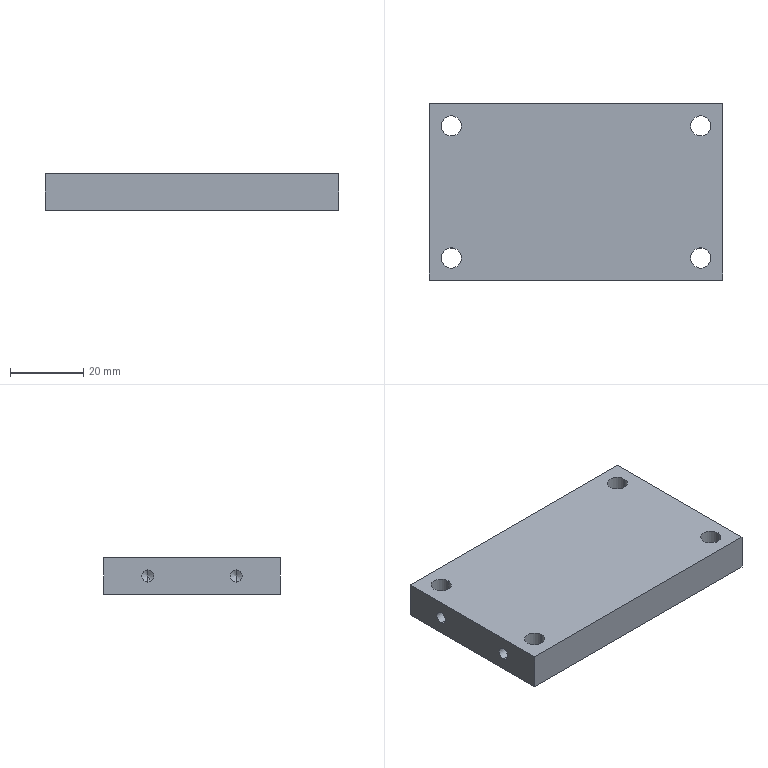Part | STEP file | B1-005 | 1 solid | 30 faces | box 80 x 48 x 10 mm | volume 37093 mm3 | cylinder 16 | cone 8 | plane 6 | commonest cylinder face diameters 3.3 x8 5.5 x8